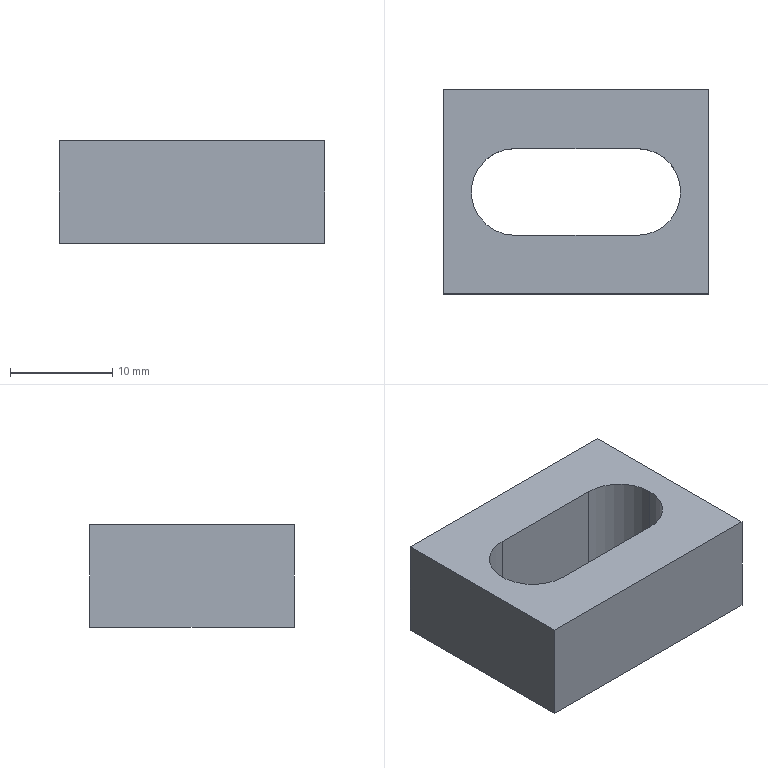Part | NX | 1 solid | 11 faces | box 26 x 20 x 10 mm | volume 3613 mm3 | plane 8 | cylinder 3 | commonest cylinder face diameters 8.5 x3
STEP:
#1=CARTESIAN_POINT('',(0.,-20.,0.));
#2=VERTEX_POINT('',#1);
#3=CARTESIAN_POINT('',(0.,0.,0.));
#4=VERTEX_POINT('',#3);
#5=CARTESIAN_POINT('',(0.,-20.,0.));
#6=DIRECTION('',(0.,1.,0.));
#7=VECTOR('',#6,1000.);
#8=LINE('',#5,#7);
#9=EDGE_CURVE('',#2,#4,#8,.T.);
#10=ORIENTED_EDGE('',*,*,#9,.T.);
#11=CARTESIAN_POINT('',(26.,0.,0.));
#12=VERTEX_POINT('',#11);
#13=CARTESIAN_POINT('',(0.,0.,0.));
#14=DIRECTION('',(1.,0.,0.));
#15=VECTOR('',#14,1000.);
#16=LINE('',#13,#15);
#17=EDGE_CURVE('',#4,#12,#16,.T.);
#18=ORIENTED_EDGE('',*,*,#17,.T.);
#19=CARTESIAN_POINT('',(26.,-20.,0.));
#20=VERTEX_POINT('',#19);
#21=CARTESIAN_POINT('',(26.,0.,0.));
#22=DIRECTION('',(0.,-1.,0.));
#23=VECTOR('',#22,1000.);
#24=LINE('',#21,#23);
#25=EDGE_CURVE('',#12,#20,#24,.T.);
#26=ORIENTED_EDGE('',*,*,#25,.T.);
#27=CARTESIAN_POINT('',(26.,-20.,0.));
#28=DIRECTION('',(-1.,0.,0.));
#29=VECTOR('',#28,1000.);
#30=LINE('',#27,#29);
#31=EDGE_CURVE('',#20,#2,#30,.T.);
#32=ORIENTED_EDGE('',*,*,#31,.T.);
#33=EDGE_LOOP('',(#10,#18,#26,#32));
#34=FACE_BOUND('',#33,.T.);
#35=CARTESIAN_POINT('',(7.,-14.25,0.));
#36=VERTEX_POINT('',#35);
#37=CARTESIAN_POINT('',(7.,-5.75,0.));
#38=VERTEX_POINT('',#37);
#39=CARTESIAN_POINT('',(7.,-10.,0.));
#40=DIRECTION('',(0.,0.,-1.));
#41=DIRECTION('',(-1.,0.,0.));
#42=AXIS2_PLACEMENT_3D('',#39,#40,#41);
#43=CIRCLE('',#42,4.25);
#44=EDGE_CURVE('',#36,#38,#43,.T.);
#45=ORIENTED_EDGE('',*,*,#44,.F.);
#46=CARTESIAN_POINT('',(19.,-14.25,0.));
#47=VERTEX_POINT('',#46);
#48=CARTESIAN_POINT('',(19.,-14.25,0.));
#49=DIRECTION('',(-1.,0.,0.));
#50=VECTOR('',#49,1000.);
#51=LINE('',#48,#50);
#52=EDGE_CURVE('',#47,#36,#51,.T.);
#53=ORIENTED_EDGE('',*,*,#52,.F.);
#54=CARTESIAN_POINT('',(23.25,-10.,0.));
#55=VERTEX_POINT('',#54);
#56=CARTESIAN_POINT('',(19.,-10.,0.));
#57=DIRECTION('',(0.,0.,-1.));
#58=DIRECTION('',(1.,0.,0.));
#59=AXIS2_PLACEMENT_3D('',#56,#57,#58);
#60=CIRCLE('',#59,4.25);
#61=EDGE_CURVE('',#55,#47,#60,.T.);
#62=ORIENTED_EDGE('',*,*,#61,.F.);
#63=CARTESIAN_POINT('',(19.,-5.75,0.));
#64=VERTEX_POINT('',#63);
#65=CARTESIAN_POINT('',(19.,-10.,0.));
#66=DIRECTION('',(0.,0.,-1.));
#67=DIRECTION('',(1.,0.,0.));
#68=AXIS2_PLACEMENT_3D('',#65,#66,#67);
#69=CIRCLE('',#68,4.25);
#70=EDGE_CURVE('',#64,#55,#69,.T.);
#71=ORIENTED_EDGE('',*,*,#70,.F.);
#72=CARTESIAN_POINT('',(7.,-5.75,0.));
#73=DIRECTION('',(1.,0.,0.));
#74=VECTOR('',#73,1000.);
#75=LINE('',#72,#74);
#76=EDGE_CURVE('',#38,#64,#75,.T.);
#77=ORIENTED_EDGE('',*,*,#76,.F.);
#78=EDGE_LOOP('',(#45,#53,#62,#71,#77));
#79=FACE_BOUND('',#78,.T.);
#80=CARTESIAN_POINT('',(0.,0.,0.));
#81=DIRECTION('',(0.,0.,1.));
#82=DIRECTION('',(1.,0.,0.));
#83=AXIS2_PLACEMENT_3D('',#80,#81,#82);
#84=PLANE('',#83);
#85=ADVANCED_FACE('',(#34,#79),#84,.F.);
#86=ORIENTED_EDGE('',*,*,#9,.F.);
#87=CARTESIAN_POINT('',(0.,-20.,10.));
#88=VERTEX_POINT('',#87);
#89=CARTESIAN_POINT('',(0.,-20.,10.));
#90=DIRECTION('',(0.,0.,-1.));
#91=VECTOR('',#90,1000.);
#92=LINE('',#89,#91);
#93=EDGE_CURVE('',#88,#2,#92,.T.);
#94=ORIENTED_EDGE('',*,*,#93,.F.);
#95=CARTESIAN_POINT('',(0.,0.,10.));
#96=VERTEX_POINT('',#95);
#97=CARTESIAN_POINT('',(0.,-20.,10.));
#98=DIRECTION('',(0.,1.,0.));
#99=VECTOR('',#98,1000.);
#100=LINE('',#97,#99);
#101=EDGE_CURVE('',#88,#96,#100,.T.);
#102=ORIENTED_EDGE('',*,*,#101,.T.);
#103=CARTESIAN_POINT('',(0.,0.,10.));
#104=DIRECTION('',(0.,0.,-1.));
#105=VECTOR('',#104,1000.);
#106=LINE('',#103,#105);
#107=EDGE_CURVE('',#96,#4,#106,.T.);
#108=ORIENTED_EDGE('',*,*,#107,.T.);
#109=EDGE_LOOP('',(#86,#94,#102,#108));
#110=FACE_BOUND('',#109,.T.);
#111=CARTESIAN_POINT('',(0.,0.,0.));
#112=DIRECTION('',(-1.,0.,0.));
#113=DIRECTION('',(0.,0.,1.));
#114=AXIS2_PLACEMENT_3D('',#111,#112,#113);
#115=PLANE('',#114);
#116=ADVANCED_FACE('',(#110),#115,.T.);
#117=ORIENTED_EDGE('',*,*,#17,.F.);
#118=ORIENTED_EDGE('',*,*,#107,.F.);
#119=CARTESIAN_POINT('',(26.,0.,10.));
#120=VERTEX_POINT('',#119);
#121=CARTESIAN_POINT('',(0.,0.,10.));
#122=DIRECTION('',(1.,0.,0.));
#123=VECTOR('',#122,1000.);
#124=LINE('',#121,#123);
#125=EDGE_CURVE('',#96,#120,#124,.T.);
#126=ORIENTED_EDGE('',*,*,#125,.T.);
#127=CARTESIAN_POINT('',(26.,0.,10.));
#128=DIRECTION('',(0.,0.,-1.));
#129=VECTOR('',#128,1000.);
#130=LINE('',#127,#129);
#131=EDGE_CURVE('',#120,#12,#130,.T.);
#132=ORIENTED_EDGE('',*,*,#131,.T.);
#133=EDGE_LOOP('',(#117,#118,#126,#132));
#134=FACE_BOUND('',#133,.T.);
#135=CARTESIAN_POINT('',(26.,0.,0.));
#136=DIRECTION('',(0.,1.,0.));
#137=DIRECTION('',(1.,0.,0.));
#138=AXIS2_PLACEMENT_3D('',#135,#136,#137);
#139=PLANE('',#138);
#140=ADVANCED_FACE('',(#134),#139,.T.);
#141=ORIENTED_EDGE('',*,*,#25,.F.);
#142=ORIENTED_EDGE('',*,*,#131,.F.);
#143=CARTESIAN_POINT('',(26.,-20.,10.));
#144=VERTEX_POINT('',#143);
#145=CARTESIAN_POINT('',(26.,0.,10.));
#146=DIRECTION('',(0.,-1.,0.));
#147=VECTOR('',#146,1000.);
#148=LINE('',#145,#147);
#149=EDGE_CURVE('',#120,#144,#148,.T.);
#150=ORIENTED_EDGE('',*,*,#149,.T.);
#151=CARTESIAN_POINT('',(26.,-20.,10.));
#152=DIRECTION('',(0.,0.,-1.));
#153=VECTOR('',#152,1000.);
#154=LINE('',#151,#153);
#155=EDGE_CURVE('',#144,#20,#154,.T.);
#156=ORIENTED_EDGE('',*,*,#155,.T.);
#157=EDGE_LOOP('',(#141,#142,#150,#156));
#158=FACE_BOUND('',#157,.T.);
#159=CARTESIAN_POINT('',(26.,-20.,0.));
#160=DIRECTION('',(1.,0.,0.));
#161=DIRECTION('',(0.,1.,0.));
#162=AXIS2_PLACEMENT_3D('',#159,#160,#161);
#163=PLANE('',#162);
#164=ADVANCED_FACE('',(#158),#163,.T.);
#165=ORIENTED_EDGE('',*,*,#31,.F.);
#166=ORIENTED_EDGE('',*,*,#155,.F.);
#167=CARTESIAN_POINT('',(26.,-20.,10.));
#168=DIRECTION('',(-1.,0.,0.));
#169=VECTOR('',#168,1000.);
#170=LINE('',#167,#169);
#171=EDGE_CURVE('',#144,#88,#170,.T.);
#172=ORIENTED_EDGE('',*,*,#171,.T.);
#173=ORIENTED_EDGE('',*,*,#93,.T.);
#174=EDGE_LOOP('',(#165,#166,#172,#173));
#175=FACE_BOUND('',#174,.T.);
#176=CARTESIAN_POINT('',(0.,-20.,0.));
#177=DIRECTION('',(0.,-1.,0.));
#178=DIRECTION('',(0.,0.,-1.));
#179=AXIS2_PLACEMENT_3D('',#176,#177,#178);
#180=PLANE('',#179);
#181=ADVANCED_FACE('',(#175),#180,.T.);
#182=ORIENTED_EDGE('',*,*,#101,.F.);
#183=ORIENTED_EDGE('',*,*,#171,.F.);
#184=ORIENTED_EDGE('',*,*,#149,.F.);
#185=ORIENTED_EDGE('',*,*,#125,.F.);
#186=EDGE_LOOP('',(#182,#183,#184,#185));
#187=FACE_BOUND('',#186,.T.);
#188=CARTESIAN_POINT('',(7.,-5.75,10.));
#189=VERTEX_POINT('',#188);
#190=CARTESIAN_POINT('',(7.,-14.25,10.));
#191=VERTEX_POINT('',#190);
#192=CARTESIAN_POINT('',(7.,-10.,10.));
#193=DIRECTION('',(0.,0.,1.));
#194=DIRECTION('',(-1.,0.,0.));
#195=AXIS2_PLACEMENT_3D('',#192,#193,#194);
#196=CIRCLE('',#195,4.25);
#197=EDGE_CURVE('',#189,#191,#196,.T.);
#198=ORIENTED_EDGE('',*,*,#197,.F.);
#199=CARTESIAN_POINT('',(19.,-5.75,10.));
#200=VERTEX_POINT('',#199);
#201=CARTESIAN_POINT('',(7.,-5.75,10.));
#202=DIRECTION('',(1.,0.,0.));
#203=VECTOR('',#202,1000.);
#204=LINE('',#201,#203);
#205=EDGE_CURVE('',#189,#200,#204,.T.);
#206=ORIENTED_EDGE('',*,*,#205,.T.);
#207=CARTESIAN_POINT('',(23.25,-10.,10.));
#208=VERTEX_POINT('',#207);
#209=CARTESIAN_POINT('',(19.,-10.,10.));
#210=DIRECTION('',(0.,0.,1.));
#211=DIRECTION('',(1.,0.,0.));
#212=AXIS2_PLACEMENT_3D('',#209,#210,#211);
#213=CIRCLE('',#212,4.25);
#214=EDGE_CURVE('',#208,#200,#213,.T.);
#215=ORIENTED_EDGE('',*,*,#214,.F.);
#216=CARTESIAN_POINT('',(19.,-14.25,10.));
#217=VERTEX_POINT('',#216);
#218=CARTESIAN_POINT('',(19.,-10.,10.));
#219=DIRECTION('',(0.,0.,1.));
#220=DIRECTION('',(1.,0.,0.));
#221=AXIS2_PLACEMENT_3D('',#218,#219,#220);
#222=CIRCLE('',#221,4.25);
#223=EDGE_CURVE('',#217,#208,#222,.T.);
#224=ORIENTED_EDGE('',*,*,#223,.F.);
#225=CARTESIAN_POINT('',(19.,-14.25,10.));
#226=DIRECTION('',(-1.,0.,0.));
#227=VECTOR('',#226,1000.);
#228=LINE('',#225,#227);
#229=EDGE_CURVE('',#217,#191,#228,.T.);
#230=ORIENTED_EDGE('',*,*,#229,.T.);
#231=EDGE_LOOP('',(#198,#206,#215,#224,#230));
#232=FACE_BOUND('',#231,.T.);
#233=CARTESIAN_POINT('',(0.,0.,10.));
#234=DIRECTION('',(0.,0.,1.));
#235=DIRECTION('',(1.,0.,0.));
#236=AXIS2_PLACEMENT_3D('',#233,#234,#235);
#237=PLANE('',#236);
#238=ADVANCED_FACE('',(#187,#232),#237,.T.);
#239=ORIENTED_EDGE('',*,*,#44,.T.);
#240=CARTESIAN_POINT('',(7.,-5.75,10.));
#241=DIRECTION('',(0.,0.,-1.));
#242=VECTOR('',#241,1000.);
#243=LINE('',#240,#242);
#244=EDGE_CURVE('',#189,#38,#243,.T.);
#245=ORIENTED_EDGE('',*,*,#244,.F.);
#246=ORIENTED_EDGE('',*,*,#197,.T.);
#247=CARTESIAN_POINT('',(7.,-14.25,0.));
#248=DIRECTION('',(0.,0.,1.));
#249=VECTOR('',#248,1000.);
#250=LINE('',#247,#249);
#251=EDGE_CURVE('',#36,#191,#250,.T.);
#252=ORIENTED_EDGE('',*,*,#251,.F.);
#253=EDGE_LOOP('',(#239,#245,#246,#252));
#254=FACE_BOUND('',#253,.T.);
#255=CARTESIAN_POINT('',(7.,-10.,10.));
#256=DIRECTION('',(0.,0.,1.));
#257=DIRECTION('',(1.,0.,0.));
#258=AXIS2_PLACEMENT_3D('',#255,#256,#257);
#259=CYLINDRICAL_SURFACE('',#258,4.25);
#260=ADVANCED_FACE('',(#254),#259,.F.);
#261=ORIENTED_EDGE('',*,*,#52,.T.);
#262=ORIENTED_EDGE('',*,*,#251,.T.);
#263=ORIENTED_EDGE('',*,*,#229,.F.);
#264=CARTESIAN_POINT('',(19.,-14.25,10.));
#265=DIRECTION('',(0.,0.,-1.));
#266=VECTOR('',#265,1000.);
#267=LINE('',#264,#266);
#268=EDGE_CURVE('',#217,#47,#267,.T.);
#269=ORIENTED_EDGE('',*,*,#268,.T.);
#270=EDGE_LOOP('',(#261,#262,#263,#269));
#271=FACE_BOUND('',#270,.T.);
#272=CARTESIAN_POINT('',(7.,-14.25,10.));
#273=DIRECTION('',(0.,-1.,0.));
#274=DIRECTION('',(0.,0.,-1.));
#275=AXIS2_PLACEMENT_3D('',#272,#273,#274);
#276=PLANE('',#275);
#277=ADVANCED_FACE('',(#271),#276,.F.);
#278=CARTESIAN_POINT('',(23.25,-10.,10.));
#279=DIRECTION('',(0.,0.,1.));
#280=VECTOR('',#279,1000.);
#281=LINE('',#278,#280);
#282=EDGE_CURVE('',#55,#208,#281,.T.);
#283=ORIENTED_EDGE('',*,*,#282,.F.);
#284=ORIENTED_EDGE('',*,*,#61,.T.);
#285=ORIENTED_EDGE('',*,*,#268,.F.);
#286=ORIENTED_EDGE('',*,*,#223,.T.);
#287=EDGE_LOOP('',(#283,#284,#285,#286));
#288=FACE_BOUND('',#287,.T.);
#289=CARTESIAN_POINT('',(19.,-10.,10.));
#290=DIRECTION('',(0.,0.,1.));
#291=DIRECTION('',(1.,0.,0.));
#292=AXIS2_PLACEMENT_3D('',#289,#290,#291);
#293=CYLINDRICAL_SURFACE('',#292,4.25);
#294=ADVANCED_FACE('',(#288),#293,.F.);
#295=ORIENTED_EDGE('',*,*,#76,.T.);
#296=CARTESIAN_POINT('',(19.,-5.75,0.));
#297=DIRECTION('',(0.,0.,1.));
#298=VECTOR('',#297,1000.);
#299=LINE('',#296,#298);
#300=EDGE_CURVE('',#64,#200,#299,.T.);
#301=ORIENTED_EDGE('',*,*,#300,.T.);
#302=ORIENTED_EDGE('',*,*,#205,.F.);
#303=ORIENTED_EDGE('',*,*,#244,.T.);
#304=EDGE_LOOP('',(#295,#301,#302,#303));
#305=FACE_BOUND('',#304,.T.);
#306=CARTESIAN_POINT('',(19.,-5.75,10.));
#307=DIRECTION('',(0.,1.,0.));
#308=DIRECTION('',(1.,0.,0.));
#309=AXIS2_PLACEMENT_3D('',#306,#307,#308);
#310=PLANE('',#309);
#311=ADVANCED_FACE('',(#305),#310,.F.);
#312=ORIENTED_EDGE('',*,*,#70,.T.);
#313=ORIENTED_EDGE('',*,*,#282,.T.);
#314=ORIENTED_EDGE('',*,*,#214,.T.);
#315=ORIENTED_EDGE('',*,*,#300,.F.);
#316=EDGE_LOOP('',(#312,#313,#314,#315));
#317=FACE_BOUND('',#316,.T.);
#318=CARTESIAN_POINT('',(19.,-10.,10.));
#319=DIRECTION('',(0.,0.,1.));
#320=DIRECTION('',(1.,0.,0.));
#321=AXIS2_PLACEMENT_3D('',#318,#319,#320);
#322=CYLINDRICAL_SURFACE('',#321,4.25);
#323=ADVANCED_FACE('',(#317),#322,.F.);
#324=CLOSED_SHELL('',(#85,#116,#140,#164,#181,#238,#260,#277,#294,#311,#323));
#325=MANIFOLD_SOLID_BREP('',#324);
#326=(LENGTH_UNIT()NAMED_UNIT(*)SI_UNIT(.MILLI.,.METRE.));
#327=UNCERTAINTY_MEASURE_WITH_UNIT(LENGTH_MEASURE(0.00001),#326,'','');
#328=(NAMED_UNIT(*)PLANE_ANGLE_UNIT()SI_UNIT($,.RADIAN.));
#329=(NAMED_UNIT(*)SI_UNIT($,.STERADIAN.)SOLID_ANGLE_UNIT());
#330=(GEOMETRIC_REPRESENTATION_CONTEXT(3)GLOBAL_UNCERTAINTY_ASSIGNED_CONTEXT((#327))GLOBAL_UNIT_ASSIGNED_CONTEXT((#326,#328,#329))REPRESENTATION_CONTEXT('',''));
#331=ADVANCED_BREP_SHAPE_REPRESENTATION('',(#325),#330);